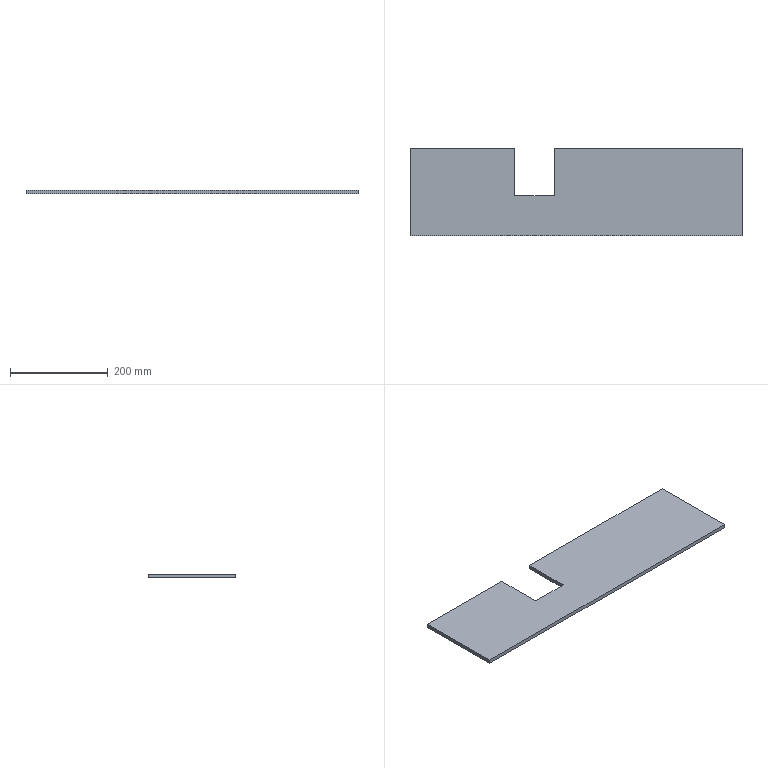Part | STEP file | 06-Steel plate 680x180x8 | 1 solid | 10 faces | box 680 x 180 x 8 mm | volume 916480 mm3 | plane 10
STEP:
#1=CARTESIAN_POINT('',(0.,0.,0.));
#2=DIRECTION('',(0.,0.,1.));
#3=DIRECTION('',(1.,0.,0.));
#4=AXIS2_PLACEMENT_3D('',#1,#2,#3);
#5=CARTESIAN_POINT('',(0.,0.,0.));
#6=VERTEX_POINT('',#5);
#7=CARTESIAN_POINT('',(0.,-180.,0.));
#8=VERTEX_POINT('',#7);
#9=CARTESIAN_POINT('',(0.,0.,0.));
#10=DIRECTION('',(0.,-1.,0.));
#11=VECTOR('',#10,1.);
#12=LINE('',#9,#11);
#13=CARTESIAN_POINT('',(0.,0.,8.));
#14=DIRECTION('',(1.,0.,0.));
#15=DIRECTION('',(0.,1.,0.));
#16=AXIS2_PLACEMENT_3D('',#13,#14,#15);
#17=PLANE('',#16);
#18=CARTESIAN_POINT('',(0.,-8.));
#19=DIRECTION('',(-1.,0.));
#20=VECTOR('',#19,1.);
#21=LINE('',#18,#20);
#22=(GEOMETRIC_REPRESENTATION_CONTEXT(2)PARAMETRIC_REPRESENTATION_CONTEXT()REPRESENTATION_CONTEXT('',''));
#23=DEFINITIONAL_REPRESENTATION('',(#21),#22);
#24=PCURVE('',#17,#23);
#25=CARTESIAN_POINT('',(0.,0.,0.));
#26=DIRECTION('',(0.,0.,1.));
#27=DIRECTION('',(1.,0.,0.));
#28=AXIS2_PLACEMENT_3D('',#25,#26,#27);
#29=PLANE('',#28);
#30=CARTESIAN_POINT('',(0.,0.));
#31=DIRECTION('',(0.,-1.));
#32=VECTOR('',#31,1.);
#33=LINE('',#30,#32);
#34=(GEOMETRIC_REPRESENTATION_CONTEXT(2)PARAMETRIC_REPRESENTATION_CONTEXT()REPRESENTATION_CONTEXT('',''));
#35=DEFINITIONAL_REPRESENTATION('',(#33),#34);
#36=PCURVE('',#29,#35);
#37=SURFACE_CURVE('',#12,(#24,#36),.PCURVE_S1.);
#38=EDGE_CURVE('',#6,#8,#37,.T.);
#39=ORIENTED_EDGE('',*,*,#38,.T.);
#40=CARTESIAN_POINT('',(0.,-180.,8.));
#41=VERTEX_POINT('',#40);
#42=CARTESIAN_POINT('',(0.,-180.,8.));
#43=DIRECTION('',(0.,0.,-1.));
#44=VECTOR('',#43,1.);
#45=LINE('',#42,#44);
#46=CARTESIAN_POINT('',(-180.,0.));
#47=DIRECTION('',(0.,-1.));
#48=VECTOR('',#47,1.);
#49=LINE('',#46,#48);
#50=(GEOMETRIC_REPRESENTATION_CONTEXT(2)PARAMETRIC_REPRESENTATION_CONTEXT()REPRESENTATION_CONTEXT('',''));
#51=DEFINITIONAL_REPRESENTATION('',(#49),#50);
#52=PCURVE('',#17,#51);
#53=CARTESIAN_POINT('',(0.,-180.,8.));
#54=DIRECTION('',(0.,1.,0.));
#55=DIRECTION('',(0.,0.,1.));
#56=AXIS2_PLACEMENT_3D('',#53,#54,#55);
#57=PLANE('',#56);
#58=CARTESIAN_POINT('',(0.,0.));
#59=DIRECTION('',(-1.,0.));
#60=VECTOR('',#59,1.);
#61=LINE('',#58,#60);
#62=(GEOMETRIC_REPRESENTATION_CONTEXT(2)PARAMETRIC_REPRESENTATION_CONTEXT()REPRESENTATION_CONTEXT('',''));
#63=DEFINITIONAL_REPRESENTATION('',(#61),#62);
#64=PCURVE('',#57,#63);
#65=SURFACE_CURVE('',#45,(#52,#64),.PCURVE_S1.);
#66=EDGE_CURVE('',#41,#8,#65,.T.);
#67=ORIENTED_EDGE('',*,*,#66,.F.);
#68=CARTESIAN_POINT('',(0.,0.,8.));
#69=VERTEX_POINT('',#68);
#70=CARTESIAN_POINT('',(0.,0.,8.));
#71=DIRECTION('',(0.,-1.,0.));
#72=VECTOR('',#71,1.);
#73=LINE('',#70,#72);
#74=CARTESIAN_POINT('',(0.,0.));
#75=DIRECTION('',(-1.,0.));
#76=VECTOR('',#75,1.);
#77=LINE('',#74,#76);
#78=(GEOMETRIC_REPRESENTATION_CONTEXT(2)PARAMETRIC_REPRESENTATION_CONTEXT()REPRESENTATION_CONTEXT('',''));
#79=DEFINITIONAL_REPRESENTATION('',(#77),#78);
#80=PCURVE('',#17,#79);
#81=CARTESIAN_POINT('',(0.,0.,8.));
#82=DIRECTION('',(0.,0.,1.));
#83=DIRECTION('',(1.,0.,0.));
#84=AXIS2_PLACEMENT_3D('',#81,#82,#83);
#85=PLANE('',#84);
#86=CARTESIAN_POINT('',(0.,0.));
#87=DIRECTION('',(0.,-1.));
#88=VECTOR('',#87,1.);
#89=LINE('',#86,#88);
#90=(GEOMETRIC_REPRESENTATION_CONTEXT(2)PARAMETRIC_REPRESENTATION_CONTEXT()REPRESENTATION_CONTEXT('',''));
#91=DEFINITIONAL_REPRESENTATION('',(#89),#90);
#92=PCURVE('',#85,#91);
#93=SURFACE_CURVE('',#73,(#80,#92),.PCURVE_S1.);
#94=EDGE_CURVE('',#69,#41,#93,.T.);
#95=ORIENTED_EDGE('',*,*,#94,.F.);
#96=CARTESIAN_POINT('',(0.,0.,8.));
#97=DIRECTION('',(0.,0.,-1.));
#98=VECTOR('',#97,1.);
#99=LINE('',#96,#98);
#100=CARTESIAN_POINT('',(0.,0.));
#101=DIRECTION('',(0.,-1.));
#102=VECTOR('',#101,1.);
#103=LINE('',#100,#102);
#104=(GEOMETRIC_REPRESENTATION_CONTEXT(2)PARAMETRIC_REPRESENTATION_CONTEXT()REPRESENTATION_CONTEXT('',''));
#105=DEFINITIONAL_REPRESENTATION('',(#103),#104);
#106=PCURVE('',#17,#105);
#107=CARTESIAN_POINT('',(0.,0.,8.));
#108=DIRECTION('',(0.,-1.,0.));
#109=DIRECTION('',(0.,0.,-1.));
#110=AXIS2_PLACEMENT_3D('',#107,#108,#109);
#111=PLANE('',#110);
#112=CARTESIAN_POINT('',(0.,0.));
#113=DIRECTION('',(1.,0.));
#114=VECTOR('',#113,1.);
#115=LINE('',#112,#114);
#116=(GEOMETRIC_REPRESENTATION_CONTEXT(2)PARAMETRIC_REPRESENTATION_CONTEXT()REPRESENTATION_CONTEXT('',''));
#117=DEFINITIONAL_REPRESENTATION('',(#115),#116);
#118=PCURVE('',#111,#117);
#119=SURFACE_CURVE('',#99,(#106,#118),.PCURVE_S1.);
#120=EDGE_CURVE('',#69,#6,#119,.T.);
#121=ORIENTED_EDGE('',*,*,#120,.T.);
#122=EDGE_LOOP('',(#39,#67,#95,#121));
#123=FACE_BOUND('',#122,.T.);
#124=ADVANCED_FACE('',(#123),#17,.F.);
#125=CARTESIAN_POINT('',(680.,-180.,0.));
#126=VERTEX_POINT('',#125);
#127=CARTESIAN_POINT('',(0.,-180.,0.));
#128=DIRECTION('',(1.,0.,0.));
#129=VECTOR('',#128,1.);
#130=LINE('',#127,#129);
#131=CARTESIAN_POINT('',(-8.,0.));
#132=DIRECTION('',(0.,1.));
#133=VECTOR('',#132,1.);
#134=LINE('',#131,#133);
#135=(GEOMETRIC_REPRESENTATION_CONTEXT(2)PARAMETRIC_REPRESENTATION_CONTEXT()REPRESENTATION_CONTEXT('',''));
#136=DEFINITIONAL_REPRESENTATION('',(#134),#135);
#137=PCURVE('',#57,#136);
#138=CARTESIAN_POINT('',(0.,-180.));
#139=DIRECTION('',(1.,0.));
#140=VECTOR('',#139,1.);
#141=LINE('',#138,#140);
#142=(GEOMETRIC_REPRESENTATION_CONTEXT(2)PARAMETRIC_REPRESENTATION_CONTEXT()REPRESENTATION_CONTEXT('',''));
#143=DEFINITIONAL_REPRESENTATION('',(#141),#142);
#144=PCURVE('',#29,#143);
#145=SURFACE_CURVE('',#130,(#137,#144),.PCURVE_S1.);
#146=EDGE_CURVE('',#8,#126,#145,.T.);
#147=ORIENTED_EDGE('',*,*,#146,.T.);
#148=CARTESIAN_POINT('',(680.,-180.,8.));
#149=VERTEX_POINT('',#148);
#150=CARTESIAN_POINT('',(680.,-180.,8.));
#151=DIRECTION('',(0.,0.,-1.));
#152=VECTOR('',#151,1.);
#153=LINE('',#150,#152);
#154=CARTESIAN_POINT('',(0.,680.));
#155=DIRECTION('',(-1.,0.));
#156=VECTOR('',#155,1.);
#157=LINE('',#154,#156);
#158=(GEOMETRIC_REPRESENTATION_CONTEXT(2)PARAMETRIC_REPRESENTATION_CONTEXT()REPRESENTATION_CONTEXT('',''));
#159=DEFINITIONAL_REPRESENTATION('',(#157),#158);
#160=PCURVE('',#57,#159);
#161=CARTESIAN_POINT('',(680.,0.,8.));
#162=DIRECTION('',(-1.,0.,0.));
#163=DIRECTION('',(0.,-1.,0.));
#164=AXIS2_PLACEMENT_3D('',#161,#162,#163);
#165=PLANE('',#164);
#166=CARTESIAN_POINT('',(180.,0.));
#167=DIRECTION('',(0.,-1.));
#168=VECTOR('',#167,1.);
#169=LINE('',#166,#168);
#170=(GEOMETRIC_REPRESENTATION_CONTEXT(2)PARAMETRIC_REPRESENTATION_CONTEXT()REPRESENTATION_CONTEXT('',''));
#171=DEFINITIONAL_REPRESENTATION('',(#169),#170);
#172=PCURVE('',#165,#171);
#173=SURFACE_CURVE('',#153,(#160,#172),.PCURVE_S1.);
#174=EDGE_CURVE('',#149,#126,#173,.T.);
#175=ORIENTED_EDGE('',*,*,#174,.F.);
#176=CARTESIAN_POINT('',(0.,-180.,8.));
#177=DIRECTION('',(1.,0.,0.));
#178=VECTOR('',#177,1.);
#179=LINE('',#176,#178);
#180=CARTESIAN_POINT('',(0.,0.));
#181=DIRECTION('',(0.,1.));
#182=VECTOR('',#181,1.);
#183=LINE('',#180,#182);
#184=(GEOMETRIC_REPRESENTATION_CONTEXT(2)PARAMETRIC_REPRESENTATION_CONTEXT()REPRESENTATION_CONTEXT('',''));
#185=DEFINITIONAL_REPRESENTATION('',(#183),#184);
#186=PCURVE('',#57,#185);
#187=CARTESIAN_POINT('',(0.,-180.));
#188=DIRECTION('',(1.,0.));
#189=VECTOR('',#188,1.);
#190=LINE('',#187,#189);
#191=(GEOMETRIC_REPRESENTATION_CONTEXT(2)PARAMETRIC_REPRESENTATION_CONTEXT()REPRESENTATION_CONTEXT('',''));
#192=DEFINITIONAL_REPRESENTATION('',(#190),#191);
#193=PCURVE('',#85,#192);
#194=SURFACE_CURVE('',#179,(#186,#193),.PCURVE_S1.);
#195=EDGE_CURVE('',#41,#149,#194,.T.);
#196=ORIENTED_EDGE('',*,*,#195,.F.);
#197=ORIENTED_EDGE('',*,*,#66,.T.);
#198=EDGE_LOOP('',(#147,#175,#196,#197));
#199=FACE_BOUND('',#198,.T.);
#200=ADVANCED_FACE('',(#199),#57,.F.);
#201=CARTESIAN_POINT('',(680.,0.,0.));
#202=VERTEX_POINT('',#201);
#203=CARTESIAN_POINT('',(680.,0.,0.));
#204=DIRECTION('',(0.,1.,0.));
#205=VECTOR('',#204,1.);
#206=LINE('',#203,#205);
#207=CARTESIAN_POINT('',(0.,-8.));
#208=DIRECTION('',(-1.,0.));
#209=VECTOR('',#208,1.);
#210=LINE('',#207,#209);
#211=(GEOMETRIC_REPRESENTATION_CONTEXT(2)PARAMETRIC_REPRESENTATION_CONTEXT()REPRESENTATION_CONTEXT('',''));
#212=DEFINITIONAL_REPRESENTATION('',(#210),#211);
#213=PCURVE('',#165,#212);
#214=CARTESIAN_POINT('',(680.,0.));
#215=DIRECTION('',(0.,1.));
#216=VECTOR('',#215,1.);
#217=LINE('',#214,#216);
#218=(GEOMETRIC_REPRESENTATION_CONTEXT(2)PARAMETRIC_REPRESENTATION_CONTEXT()REPRESENTATION_CONTEXT('',''));
#219=DEFINITIONAL_REPRESENTATION('',(#217),#218);
#220=PCURVE('',#29,#219);
#221=SURFACE_CURVE('',#206,(#213,#220),.PCURVE_S1.);
#222=EDGE_CURVE('',#126,#202,#221,.T.);
#223=ORIENTED_EDGE('',*,*,#222,.T.);
#224=CARTESIAN_POINT('',(680.,0.,8.));
#225=VERTEX_POINT('',#224);
#226=CARTESIAN_POINT('',(680.,0.,8.));
#227=DIRECTION('',(0.,0.,-1.));
#228=VECTOR('',#227,1.);
#229=LINE('',#226,#228);
#230=CARTESIAN_POINT('',(0.,0.));
#231=DIRECTION('',(0.,-1.));
#232=VECTOR('',#231,1.);
#233=LINE('',#230,#232);
#234=(GEOMETRIC_REPRESENTATION_CONTEXT(2)PARAMETRIC_REPRESENTATION_CONTEXT()REPRESENTATION_CONTEXT('',''));
#235=DEFINITIONAL_REPRESENTATION('',(#233),#234);
#236=PCURVE('',#165,#235);
#237=CARTESIAN_POINT('',(295.,0.,8.));
#238=DIRECTION('',(0.,-1.,0.));
#239=DIRECTION('',(0.,0.,-1.));
#240=AXIS2_PLACEMENT_3D('',#237,#238,#239);
#241=PLANE('',#240);
#242=CARTESIAN_POINT('',(0.,385.));
#243=DIRECTION('',(1.,0.));
#244=VECTOR('',#243,1.);
#245=LINE('',#242,#244);
#246=(GEOMETRIC_REPRESENTATION_CONTEXT(2)PARAMETRIC_REPRESENTATION_CONTEXT()REPRESENTATION_CONTEXT('',''));
#247=DEFINITIONAL_REPRESENTATION('',(#245),#246);
#248=PCURVE('',#241,#247);
#249=SURFACE_CURVE('',#229,(#236,#248),.PCURVE_S1.);
#250=EDGE_CURVE('',#225,#202,#249,.T.);
#251=ORIENTED_EDGE('',*,*,#250,.F.);
#252=CARTESIAN_POINT('',(680.,0.,8.));
#253=DIRECTION('',(0.,1.,0.));
#254=VECTOR('',#253,1.);
#255=LINE('',#252,#254);
#256=CARTESIAN_POINT('',(0.,0.));
#257=DIRECTION('',(-1.,0.));
#258=VECTOR('',#257,1.);
#259=LINE('',#256,#258);
#260=(GEOMETRIC_REPRESENTATION_CONTEXT(2)PARAMETRIC_REPRESENTATION_CONTEXT()REPRESENTATION_CONTEXT('',''));
#261=DEFINITIONAL_REPRESENTATION('',(#259),#260);
#262=PCURVE('',#165,#261);
#263=CARTESIAN_POINT('',(680.,0.));
#264=DIRECTION('',(0.,1.));
#265=VECTOR('',#264,1.);
#266=LINE('',#263,#265);
#267=(GEOMETRIC_REPRESENTATION_CONTEXT(2)PARAMETRIC_REPRESENTATION_CONTEXT()REPRESENTATION_CONTEXT('',''));
#268=DEFINITIONAL_REPRESENTATION('',(#266),#267);
#269=PCURVE('',#85,#268);
#270=SURFACE_CURVE('',#255,(#262,#269),.PCURVE_S1.);
#271=EDGE_CURVE('',#149,#225,#270,.T.);
#272=ORIENTED_EDGE('',*,*,#271,.F.);
#273=ORIENTED_EDGE('',*,*,#174,.T.);
#274=EDGE_LOOP('',(#223,#251,#272,#273));
#275=FACE_BOUND('',#274,.T.);
#276=ADVANCED_FACE('',(#275),#165,.F.);
#277=CARTESIAN_POINT('',(295.,0.,0.));
#278=VERTEX_POINT('',#277);
#279=CARTESIAN_POINT('',(295.,0.,0.));
#280=DIRECTION('',(-1.,0.,0.));
#281=VECTOR('',#280,1.);
#282=LINE('',#279,#281);
#283=CARTESIAN_POINT('',(8.,0.));
#284=DIRECTION('',(0.,-1.));
#285=VECTOR('',#284,1.);
#286=LINE('',#283,#285);
#287=(GEOMETRIC_REPRESENTATION_CONTEXT(2)PARAMETRIC_REPRESENTATION_CONTEXT()REPRESENTATION_CONTEXT('',''));
#288=DEFINITIONAL_REPRESENTATION('',(#286),#287);
#289=PCURVE('',#241,#288);
#290=CARTESIAN_POINT('',(295.,0.));
#291=DIRECTION('',(-1.,0.));
#292=VECTOR('',#291,1.);
#293=LINE('',#290,#292);
#294=(GEOMETRIC_REPRESENTATION_CONTEXT(2)PARAMETRIC_REPRESENTATION_CONTEXT()REPRESENTATION_CONTEXT('',''));
#295=DEFINITIONAL_REPRESENTATION('',(#293),#294);
#296=PCURVE('',#29,#295);
#297=SURFACE_CURVE('',#282,(#289,#296),.PCURVE_S1.);
#298=EDGE_CURVE('',#202,#278,#297,.T.);
#299=ORIENTED_EDGE('',*,*,#298,.T.);
#300=CARTESIAN_POINT('',(295.,0.,8.));
#301=VERTEX_POINT('',#300);
#302=CARTESIAN_POINT('',(295.,0.,8.));
#303=DIRECTION('',(0.,0.,-1.));
#304=VECTOR('',#303,1.);
#305=LINE('',#302,#304);
#306=CARTESIAN_POINT('',(0.,0.));
#307=DIRECTION('',(1.,0.));
#308=VECTOR('',#307,1.);
#309=LINE('',#306,#308);
#310=(GEOMETRIC_REPRESENTATION_CONTEXT(2)PARAMETRIC_REPRESENTATION_CONTEXT()REPRESENTATION_CONTEXT('',''));
#311=DEFINITIONAL_REPRESENTATION('',(#309),#310);
#312=PCURVE('',#241,#311);
#313=CARTESIAN_POINT('',(295.,0.,8.));
#314=DIRECTION('',(1.,0.,0.));
#315=DIRECTION('',(0.,0.,-1.));
#316=AXIS2_PLACEMENT_3D('',#313,#314,#315);
#317=PLANE('',#316);
#318=CARTESIAN_POINT('',(0.,0.));
#319=DIRECTION('',(1.,0.));
#320=VECTOR('',#319,1.);
#321=LINE('',#318,#320);
#322=(GEOMETRIC_REPRESENTATION_CONTEXT(2)PARAMETRIC_REPRESENTATION_CONTEXT()REPRESENTATION_CONTEXT('',''));
#323=DEFINITIONAL_REPRESENTATION('',(#321),#322);
#324=PCURVE('',#317,#323);
#325=SURFACE_CURVE('',#305,(#312,#324),.PCURVE_S1.);
#326=EDGE_CURVE('',#301,#278,#325,.T.);
#327=ORIENTED_EDGE('',*,*,#326,.F.);
#328=CARTESIAN_POINT('',(295.,0.,8.));
#329=DIRECTION('',(-1.,0.,0.));
#330=VECTOR('',#329,1.);
#331=LINE('',#328,#330);
#332=CARTESIAN_POINT('',(0.,0.));
#333=DIRECTION('',(0.,-1.));
#334=VECTOR('',#333,1.);
#335=LINE('',#332,#334);
#336=(GEOMETRIC_REPRESENTATION_CONTEXT(2)PARAMETRIC_REPRESENTATION_CONTEXT()REPRESENTATION_CONTEXT('',''));
#337=DEFINITIONAL_REPRESENTATION('',(#335),#336);
#338=PCURVE('',#241,#337);
#339=CARTESIAN_POINT('',(295.,0.));
#340=DIRECTION('',(-1.,0.));
#341=VECTOR('',#340,1.);
#342=LINE('',#339,#341);
#343=(GEOMETRIC_REPRESENTATION_CONTEXT(2)PARAMETRIC_REPRESENTATION_CONTEXT()REPRESENTATION_CONTEXT('',''));
#344=DEFINITIONAL_REPRESENTATION('',(#342),#343);
#345=PCURVE('',#85,#344);
#346=SURFACE_CURVE('',#331,(#338,#345),.PCURVE_S1.);
#347=EDGE_CURVE('',#225,#301,#346,.T.);
#348=ORIENTED_EDGE('',*,*,#347,.F.);
#349=ORIENTED_EDGE('',*,*,#250,.T.);
#350=EDGE_LOOP('',(#299,#327,#348,#349));
#351=FACE_BOUND('',#350,.T.);
#352=ADVANCED_FACE('',(#351),#241,.F.);
#353=CARTESIAN_POINT('',(295.,-98.,0.));
#354=VERTEX_POINT('',#353);
#355=CARTESIAN_POINT('',(295.,0.,0.));
#356=DIRECTION('',(0.,-1.,0.));
#357=VECTOR('',#356,1.);
#358=LINE('',#355,#357);
#359=CARTESIAN_POINT('',(8.,0.));
#360=DIRECTION('',(0.,-1.));
#361=VECTOR('',#360,1.);
#362=LINE('',#359,#361);
#363=(GEOMETRIC_REPRESENTATION_CONTEXT(2)PARAMETRIC_REPRESENTATION_CONTEXT()REPRESENTATION_CONTEXT('',''));
#364=DEFINITIONAL_REPRESENTATION('',(#362),#363);
#365=PCURVE('',#317,#364);
#366=CARTESIAN_POINT('',(295.,0.));
#367=DIRECTION('',(0.,-1.));
#368=VECTOR('',#367,1.);
#369=LINE('',#366,#368);
#370=(GEOMETRIC_REPRESENTATION_CONTEXT(2)PARAMETRIC_REPRESENTATION_CONTEXT()REPRESENTATION_CONTEXT('',''));
#371=DEFINITIONAL_REPRESENTATION('',(#369),#370);
#372=PCURVE('',#29,#371);
#373=SURFACE_CURVE('',#358,(#365,#372),.PCURVE_S1.);
#374=EDGE_CURVE('',#278,#354,#373,.T.);
#375=ORIENTED_EDGE('',*,*,#374,.T.);
#376=CARTESIAN_POINT('',(295.,-98.,8.));
#377=VERTEX_POINT('',#376);
#378=CARTESIAN_POINT('',(295.,-98.,8.));
#379=DIRECTION('',(0.,0.,-1.));
#380=VECTOR('',#379,1.);
#381=LINE('',#378,#380);
#382=CARTESIAN_POINT('',(0.,-98.));
#383=DIRECTION('',(1.,0.));
#384=VECTOR('',#383,1.);
#385=LINE('',#382,#384);
#386=(GEOMETRIC_REPRESENTATION_CONTEXT(2)PARAMETRIC_REPRESENTATION_CONTEXT()REPRESENTATION_CONTEXT('',''));
#387=DEFINITIONAL_REPRESENTATION('',(#385),#386);
#388=PCURVE('',#317,#387);
#389=CARTESIAN_POINT('',(215.,-98.,8.));
#390=DIRECTION('',(0.,-1.,0.));
#391=DIRECTION('',(0.,0.,-1.));
#392=AXIS2_PLACEMENT_3D('',#389,#390,#391);
#393=PLANE('',#392);
#394=CARTESIAN_POINT('',(0.,80.));
#395=DIRECTION('',(1.,0.));
#396=VECTOR('',#395,1.);
#397=LINE('',#394,#396);
#398=(GEOMETRIC_REPRESENTATION_CONTEXT(2)PARAMETRIC_REPRESENTATION_CONTEXT()REPRESENTATION_CONTEXT('',''));
#399=DEFINITIONAL_REPRESENTATION('',(#397),#398);
#400=PCURVE('',#393,#399);
#401=SURFACE_CURVE('',#381,(#388,#400),.PCURVE_S1.);
#402=EDGE_CURVE('',#377,#354,#401,.T.);
#403=ORIENTED_EDGE('',*,*,#402,.F.);
#404=CARTESIAN_POINT('',(295.,0.,8.));
#405=DIRECTION('',(0.,-1.,0.));
#406=VECTOR('',#405,1.);
#407=LINE('',#404,#406);
#408=CARTESIAN_POINT('',(0.,0.));
#409=DIRECTION('',(0.,-1.));
#410=VECTOR('',#409,1.);
#411=LINE('',#408,#410);
#412=(GEOMETRIC_REPRESENTATION_CONTEXT(2)PARAMETRIC_REPRESENTATION_CONTEXT()REPRESENTATION_CONTEXT('',''));
#413=DEFINITIONAL_REPRESENTATION('',(#411),#412);
#414=PCURVE('',#317,#413);
#415=CARTESIAN_POINT('',(295.,0.));
#416=DIRECTION('',(0.,-1.));
#417=VECTOR('',#416,1.);
#418=LINE('',#415,#417);
#419=(GEOMETRIC_REPRESENTATION_CONTEXT(2)PARAMETRIC_REPRESENTATION_CONTEXT()REPRESENTATION_CONTEXT('',''));
#420=DEFINITIONAL_REPRESENTATION('',(#418),#419);
#421=PCURVE('',#85,#420);
#422=SURFACE_CURVE('',#407,(#414,#421),.PCURVE_S1.);
#423=EDGE_CURVE('',#301,#377,#422,.T.);
#424=ORIENTED_EDGE('',*,*,#423,.F.);
#425=ORIENTED_EDGE('',*,*,#326,.T.);
#426=EDGE_LOOP('',(#375,#403,#424,#425));
#427=FACE_BOUND('',#426,.T.);
#428=ADVANCED_FACE('',(#427),#317,.F.);
#429=CARTESIAN_POINT('',(215.,-98.,0.));
#430=VERTEX_POINT('',#429);
#431=CARTESIAN_POINT('',(215.,-98.,0.));
#432=DIRECTION('',(-1.,0.,0.));
#433=VECTOR('',#432,1.);
#434=LINE('',#431,#433);
#435=CARTESIAN_POINT('',(8.,0.));
#436=DIRECTION('',(0.,-1.));
#437=VECTOR('',#436,1.);
#438=LINE('',#435,#437);
#439=(GEOMETRIC_REPRESENTATION_CONTEXT(2)PARAMETRIC_REPRESENTATION_CONTEXT()REPRESENTATION_CONTEXT('',''));
#440=DEFINITIONAL_REPRESENTATION('',(#438),#439);
#441=PCURVE('',#393,#440);
#442=CARTESIAN_POINT('',(215.,-98.));
#443=DIRECTION('',(-1.,0.));
#444=VECTOR('',#443,1.);
#445=LINE('',#442,#444);
#446=(GEOMETRIC_REPRESENTATION_CONTEXT(2)PARAMETRIC_REPRESENTATION_CONTEXT()REPRESENTATION_CONTEXT('',''));
#447=DEFINITIONAL_REPRESENTATION('',(#445),#446);
#448=PCURVE('',#29,#447);
#449=SURFACE_CURVE('',#434,(#441,#448),.PCURVE_S1.);
#450=EDGE_CURVE('',#354,#430,#449,.T.);
#451=ORIENTED_EDGE('',*,*,#450,.T.);
#452=CARTESIAN_POINT('',(215.,-98.,8.));
#453=VERTEX_POINT('',#452);
#454=CARTESIAN_POINT('',(215.,-98.,8.));
#455=DIRECTION('',(0.,0.,-1.));
#456=VECTOR('',#455,1.);
#457=LINE('',#454,#456);
#458=CARTESIAN_POINT('',(0.,0.));
#459=DIRECTION('',(1.,0.));
#460=VECTOR('',#459,1.);
#461=LINE('',#458,#460);
#462=(GEOMETRIC_REPRESENTATION_CONTEXT(2)PARAMETRIC_REPRESENTATION_CONTEXT()REPRESENTATION_CONTEXT('',''));
#463=DEFINITIONAL_REPRESENTATION('',(#461),#462);
#464=PCURVE('',#393,#463);
#465=CARTESIAN_POINT('',(215.,0.,8.));
#466=DIRECTION('',(-1.,0.,0.));
#467=DIRECTION('',(0.,0.,1.));
#468=AXIS2_PLACEMENT_3D('',#465,#466,#467);
#469=PLANE('',#468);
#470=CARTESIAN_POINT('',(0.,-98.));
#471=DIRECTION('',(-1.,0.));
#472=VECTOR('',#471,1.);
#473=LINE('',#470,#472);
#474=(GEOMETRIC_REPRESENTATION_CONTEXT(2)PARAMETRIC_REPRESENTATION_CONTEXT()REPRESENTATION_CONTEXT('',''));
#475=DEFINITIONAL_REPRESENTATION('',(#473),#474);
#476=PCURVE('',#469,#475);
#477=SURFACE_CURVE('',#457,(#464,#476),.PCURVE_S1.);
#478=EDGE_CURVE('',#453,#430,#477,.T.);
#479=ORIENTED_EDGE('',*,*,#478,.F.);
#480=CARTESIAN_POINT('',(215.,-98.,8.));
#481=DIRECTION('',(-1.,0.,0.));
#482=VECTOR('',#481,1.);
#483=LINE('',#480,#482);
#484=CARTESIAN_POINT('',(0.,0.));
#485=DIRECTION('',(0.,-1.));
#486=VECTOR('',#485,1.);
#487=LINE('',#484,#486);
#488=(GEOMETRIC_REPRESENTATION_CONTEXT(2)PARAMETRIC_REPRESENTATION_CONTEXT()REPRESENTATION_CONTEXT('',''));
#489=DEFINITIONAL_REPRESENTATION('',(#487),#488);
#490=PCURVE('',#393,#489);
#491=CARTESIAN_POINT('',(215.,-98.));
#492=DIRECTION('',(-1.,0.));
#493=VECTOR('',#492,1.);
#494=LINE('',#491,#493);
#495=(GEOMETRIC_REPRESENTATION_CONTEXT(2)PARAMETRIC_REPRESENTATION_CONTEXT()REPRESENTATION_CONTEXT('',''));
#496=DEFINITIONAL_REPRESENTATION('',(#494),#495);
#497=PCURVE('',#85,#496);
#498=SURFACE_CURVE('',#483,(#490,#497),.PCURVE_S1.);
#499=EDGE_CURVE('',#377,#453,#498,.T.);
#500=ORIENTED_EDGE('',*,*,#499,.F.);
#501=ORIENTED_EDGE('',*,*,#402,.T.);
#502=EDGE_LOOP('',(#451,#479,#500,#501));
#503=FACE_BOUND('',#502,.T.);
#504=ADVANCED_FACE('',(#503),#393,.F.);
#505=CARTESIAN_POINT('',(215.,0.,0.));
#506=VERTEX_POINT('',#505);
#507=CARTESIAN_POINT('',(215.,0.,0.));
#508=DIRECTION('',(0.,1.,0.));
#509=VECTOR('',#508,1.);
#510=LINE('',#507,#509);
#511=CARTESIAN_POINT('',(-8.,0.));
#512=DIRECTION('',(0.,1.));
#513=VECTOR('',#512,1.);
#514=LINE('',#511,#513);
#515=(GEOMETRIC_REPRESENTATION_CONTEXT(2)PARAMETRIC_REPRESENTATION_CONTEXT()REPRESENTATION_CONTEXT('',''));
#516=DEFINITIONAL_REPRESENTATION('',(#514),#515);
#517=PCURVE('',#469,#516);
#518=CARTESIAN_POINT('',(215.,0.));
#519=DIRECTION('',(0.,1.));
#520=VECTOR('',#519,1.);
#521=LINE('',#518,#520);
#522=(GEOMETRIC_REPRESENTATION_CONTEXT(2)PARAMETRIC_REPRESENTATION_CONTEXT()REPRESENTATION_CONTEXT('',''));
#523=DEFINITIONAL_REPRESENTATION('',(#521),#522);
#524=PCURVE('',#29,#523);
#525=SURFACE_CURVE('',#510,(#517,#524),.PCURVE_S1.);
#526=EDGE_CURVE('',#430,#506,#525,.T.);
#527=ORIENTED_EDGE('',*,*,#526,.T.);
#528=CARTESIAN_POINT('',(215.,0.,8.));
#529=VERTEX_POINT('',#528);
#530=CARTESIAN_POINT('',(215.,0.,8.));
#531=DIRECTION('',(0.,0.,-1.));
#532=VECTOR('',#531,1.);
#533=LINE('',#530,#532);
#534=CARTESIAN_POINT('',(0.,0.));
#535=DIRECTION('',(-1.,0.));
#536=VECTOR('',#535,1.);
#537=LINE('',#534,#536);
#538=(GEOMETRIC_REPRESENTATION_CONTEXT(2)PARAMETRIC_REPRESENTATION_CONTEXT()REPRESENTATION_CONTEXT('',''));
#539=DEFINITIONAL_REPRESENTATION('',(#537),#538);
#540=PCURVE('',#469,#539);
#541=CARTESIAN_POINT('',(0.,215.));
#542=DIRECTION('',(1.,0.));
#543=VECTOR('',#542,1.);
#544=LINE('',#541,#543);
#545=(GEOMETRIC_REPRESENTATION_CONTEXT(2)PARAMETRIC_REPRESENTATION_CONTEXT()REPRESENTATION_CONTEXT('',''));
#546=DEFINITIONAL_REPRESENTATION('',(#544),#545);
#547=PCURVE('',#111,#546);
#548=SURFACE_CURVE('',#533,(#540,#547),.PCURVE_S1.);
#549=EDGE_CURVE('',#529,#506,#548,.T.);
#550=ORIENTED_EDGE('',*,*,#549,.F.);
#551=CARTESIAN_POINT('',(215.,0.,8.));
#552=DIRECTION('',(0.,1.,0.));
#553=VECTOR('',#552,1.);
#554=LINE('',#551,#553);
#555=CARTESIAN_POINT('',(0.,0.));
#556=DIRECTION('',(0.,1.));
#557=VECTOR('',#556,1.);
#558=LINE('',#555,#557);
#559=(GEOMETRIC_REPRESENTATION_CONTEXT(2)PARAMETRIC_REPRESENTATION_CONTEXT()REPRESENTATION_CONTEXT('',''));
#560=DEFINITIONAL_REPRESENTATION('',(#558),#559);
#561=PCURVE('',#469,#560);
#562=CARTESIAN_POINT('',(215.,0.));
#563=DIRECTION('',(0.,1.));
#564=VECTOR('',#563,1.);
#565=LINE('',#562,#564);
#566=(GEOMETRIC_REPRESENTATION_CONTEXT(2)PARAMETRIC_REPRESENTATION_CONTEXT()REPRESENTATION_CONTEXT('',''));
#567=DEFINITIONAL_REPRESENTATION('',(#565),#566);
#568=PCURVE('',#85,#567);
#569=SURFACE_CURVE('',#554,(#561,#568),.PCURVE_S1.);
#570=EDGE_CURVE('',#453,#529,#569,.T.);
#571=ORIENTED_EDGE('',*,*,#570,.F.);
#572=ORIENTED_EDGE('',*,*,#478,.T.);
#573=EDGE_LOOP('',(#527,#550,#571,#572));
#574=FACE_BOUND('',#573,.T.);
#575=ADVANCED_FACE('',(#574),#469,.F.);
#576=CARTESIAN_POINT('',(0.,0.,0.));
#577=DIRECTION('',(-1.,0.,0.));
#578=VECTOR('',#577,1.);
#579=LINE('',#576,#578);
#580=CARTESIAN_POINT('',(8.,0.));
#581=DIRECTION('',(0.,-1.));
#582=VECTOR('',#581,1.);
#583=LINE('',#580,#582);
#584=(GEOMETRIC_REPRESENTATION_CONTEXT(2)PARAMETRIC_REPRESENTATION_CONTEXT()REPRESENTATION_CONTEXT('',''));
#585=DEFINITIONAL_REPRESENTATION('',(#583),#584);
#586=PCURVE('',#111,#585);
#587=CARTESIAN_POINT('',(0.,0.));
#588=DIRECTION('',(-1.,0.));
#589=VECTOR('',#588,1.);
#590=LINE('',#587,#589);
#591=(GEOMETRIC_REPRESENTATION_CONTEXT(2)PARAMETRIC_REPRESENTATION_CONTEXT()REPRESENTATION_CONTEXT('',''));
#592=DEFINITIONAL_REPRESENTATION('',(#590),#591);
#593=PCURVE('',#29,#592);
#594=SURFACE_CURVE('',#579,(#586,#593),.PCURVE_S1.);
#595=EDGE_CURVE('',#506,#6,#594,.T.);
#596=ORIENTED_EDGE('',*,*,#595,.T.);
#597=ORIENTED_EDGE('',*,*,#120,.F.);
#598=CARTESIAN_POINT('',(0.,0.,8.));
#599=DIRECTION('',(-1.,0.,0.));
#600=VECTOR('',#599,1.);
#601=LINE('',#598,#600);
#602=CARTESIAN_POINT('',(0.,0.));
#603=DIRECTION('',(0.,-1.));
#604=VECTOR('',#603,1.);
#605=LINE('',#602,#604);
#606=(GEOMETRIC_REPRESENTATION_CONTEXT(2)PARAMETRIC_REPRESENTATION_CONTEXT()REPRESENTATION_CONTEXT('',''));
#607=DEFINITIONAL_REPRESENTATION('',(#605),#606);
#608=PCURVE('',#111,#607);
#609=CARTESIAN_POINT('',(0.,0.));
#610=DIRECTION('',(-1.,0.));
#611=VECTOR('',#610,1.);
#612=LINE('',#609,#611);
#613=(GEOMETRIC_REPRESENTATION_CONTEXT(2)PARAMETRIC_REPRESENTATION_CONTEXT()REPRESENTATION_CONTEXT('',''));
#614=DEFINITIONAL_REPRESENTATION('',(#612),#613);
#615=PCURVE('',#85,#614);
#616=SURFACE_CURVE('',#601,(#608,#615),.PCURVE_S1.);
#617=EDGE_CURVE('',#529,#69,#616,.T.);
#618=ORIENTED_EDGE('',*,*,#617,.F.);
#619=ORIENTED_EDGE('',*,*,#549,.T.);
#620=EDGE_LOOP('',(#596,#597,#618,#619));
#621=FACE_BOUND('',#620,.T.);
#622=ADVANCED_FACE('',(#621),#111,.F.);
#623=ORIENTED_EDGE('',*,*,#94,.T.);
#624=ORIENTED_EDGE('',*,*,#195,.T.);
#625=ORIENTED_EDGE('',*,*,#271,.T.);
#626=ORIENTED_EDGE('',*,*,#347,.T.);
#627=ORIENTED_EDGE('',*,*,#423,.T.);
#628=ORIENTED_EDGE('',*,*,#499,.T.);
#629=ORIENTED_EDGE('',*,*,#570,.T.);
#630=ORIENTED_EDGE('',*,*,#617,.T.);
#631=EDGE_LOOP('',(#623,#624,#625,#626,#627,#628,#629,#630));
#632=FACE_BOUND('',#631,.T.);
#633=ADVANCED_FACE('',(#632),#85,.T.);
#634=ORIENTED_EDGE('',*,*,#38,.F.);
#635=ORIENTED_EDGE('',*,*,#595,.F.);
#636=ORIENTED_EDGE('',*,*,#526,.F.);
#637=ORIENTED_EDGE('',*,*,#450,.F.);
#638=ORIENTED_EDGE('',*,*,#374,.F.);
#639=ORIENTED_EDGE('',*,*,#298,.F.);
#640=ORIENTED_EDGE('',*,*,#222,.F.);
#641=ORIENTED_EDGE('',*,*,#146,.F.);
#642=EDGE_LOOP('',(#634,#635,#636,#637,#638,#639,#640,#641));
#643=FACE_BOUND('',#642,.T.);
#644=ADVANCED_FACE('',(#643),#29,.F.);
#645=CLOSED_SHELL('',(#124,#200,#276,#352,#428,#504,#575,#622,#633,#644));
#646=MANIFOLD_SOLID_BREP('',#645);
#647=(LENGTH_UNIT()NAMED_UNIT(*)SI_UNIT(.MILLI.,.METRE.));
#648=UNCERTAINTY_MEASURE_WITH_UNIT(LENGTH_MEASURE(0.0000001),#647,'','');
#649=(NAMED_UNIT(*)PLANE_ANGLE_UNIT()SI_UNIT($,.RADIAN.));
#650=(NAMED_UNIT(*)SI_UNIT($,.STERADIAN.)SOLID_ANGLE_UNIT());
#651=(GEOMETRIC_REPRESENTATION_CONTEXT(3)GLOBAL_UNCERTAINTY_ASSIGNED_CONTEXT((#648))GLOBAL_UNIT_ASSIGNED_CONTEXT((#647,#649,#650))REPRESENTATION_CONTEXT('',''));
#652=ADVANCED_BREP_SHAPE_REPRESENTATION('',(#4,#646),#651);